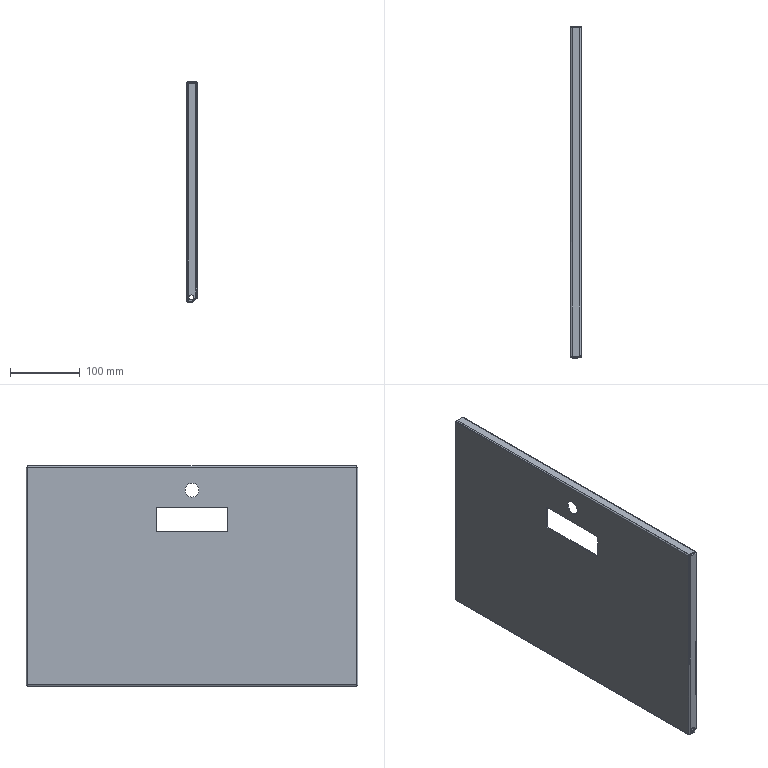Part | SolidWorks | features EdgeFlange 4, ICE 4, FlatPattern 1, SMBaseFlange 1, SheetMetal 1 | 1 solid | 92 faces | box 15 x 477 x 317 mm | volume 269673 mm3 | plane 62 | cylinder 22 | spline 8 | commonest cylinder face diameters 0.6 x7 3.6 x7 7 x4 20 x2 1.473 x1 4.473 x1